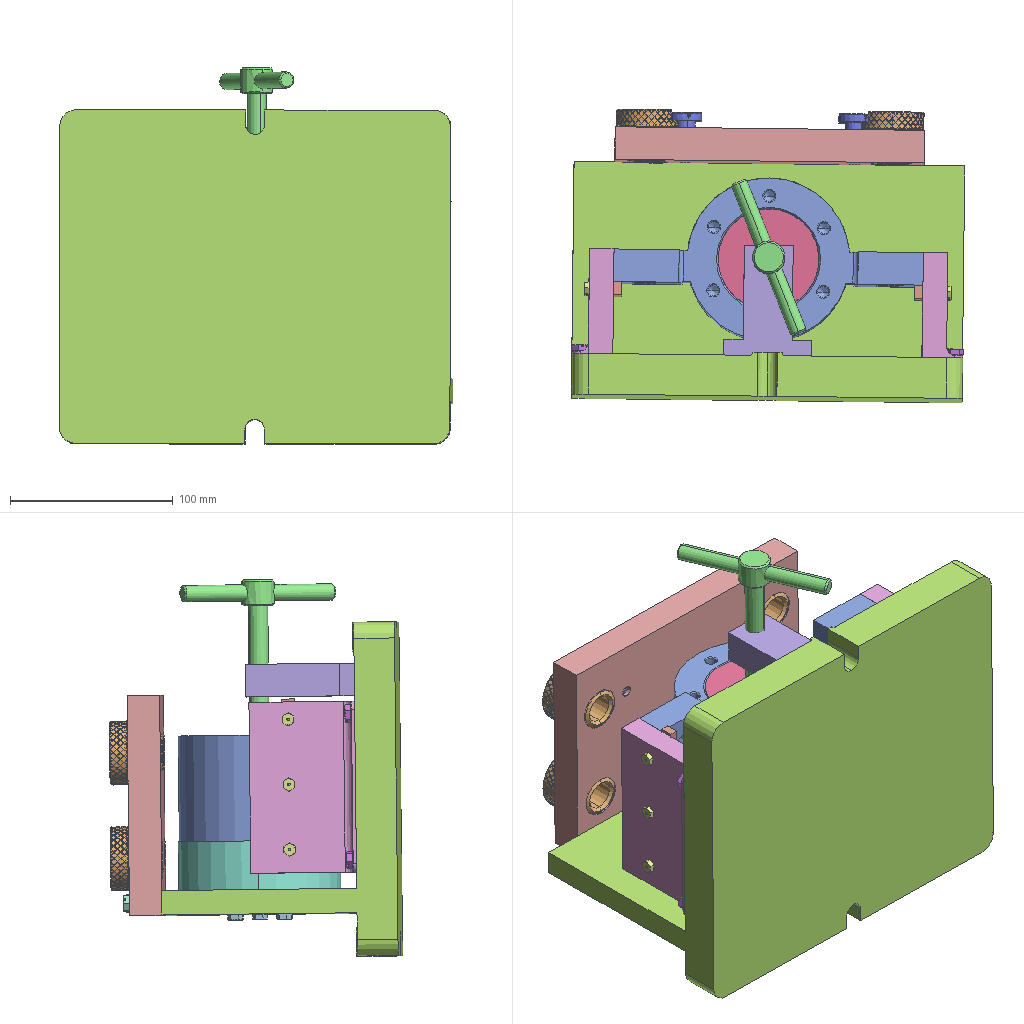Assembly | SolidWorks | 15 different items | 36 placed | box 242 x 180 x 231 mm
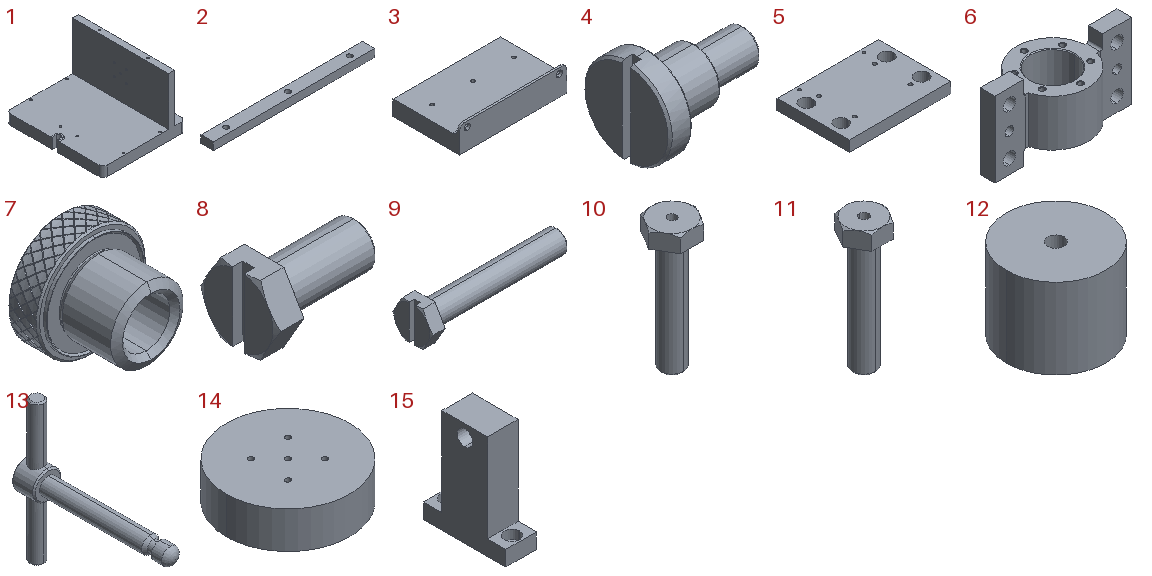Parts list (item | quantity | size | volume | features):
1 | x1 | 205 x 240 x 145 mm | 1648733 mm3 | features HoleWzd 4, Fillet 2, ICE 2, Extrusion 1
2 | x2 | 105 x 8 x 5 mm | 4072 mm3 | features Extrusion 1, HoleWzd 1
3 | x2 | 105 x 65 x 24.968 mm | 104629 mm3 | features Fillet 2, Extrusion 1, HoleWzd 1, ICE 1
4 | x4 | 27 x 20 x 20 mm | 3212 mm3 | features Chamfer 1, Fillet 1, ICE 1, Revolution 1
5 | x1 | 190 x 135 x 20 mm | 469337 mm3 | features HoleWzd 2, Extrusion 1
6 | x1 | 190 x 100 x 105 mm | 479131 mm3 | features ICE 7, Attribute 3, HoleWzd 2, Chamfer 1, Extrusion 1
7 | x4 | 39 x 32 x 39 mm | 16208 mm3 | features Chamfer 2, BlendCut 1, CirPattern 1, ICE 1, MirrorPattern 1, Revolution 1
8 | x4 | 16 x 10.9 x 9.44 mm | 614.542 mm3 | features Cut 2, Chamfer 1, Extrusion 1, Fillet 1, LPattern 1, MoveCopyBody 1, RevCut 1, Revolution 1
9 | x2 | 39 x 10.9 x 9.44 mm | 1265 mm3 | features Cut 2, Chamfer 1, Extrusion 1, Fillet 1, LPattern 1, MoveCopyBody 1, RevCut 1, Revolution 1
10 | x6 | 8.083 x 7 x 22.8 mm | 328.465 mm3 | features ICE 2, Chamfer 1, Revolution 1
11 | x5 | 9.238 x 8 x 28.5 mm | 592.822 mm3 | features ICE 2, Chamfer 1, Revolution 1
12 | x1 | 62 x 62 x 50 mm | 148480 mm3 | features Extrusion 1, HoleWzd 1
13 | x1 | 20 x 106 x 100 mm | 20892 mm3 | features Revolution 5, Chamfer 4, Dome 3
14 | x1 | 100 x 100 x 30 mm | 233541 mm3 | features Extrusion 1, HoleWzd 1
15 | x1 | 20 x 54 x 68 mm | 42750 mm3 | features HoleWzd 2, Extrusion 1, ICE 1
Mates (type | each side: item.copy, entity, surface, feature):
Concentric | 1.1 face cylinder M6 Tapped Hole3 | 3.1 face cylinder Boss-Extrude3 | 2 times
Coincident | 1.1 face plane Boss-Extrude1 | 3.1 face plane Boss-Extrude2
Concentric | 1.1 face cylinder M6 Tapped Hole3 | 3.2 face cylinder Boss-Extrude3 | 2 times
Coincident | 1.1 face plane Boss-Extrude1 | 3.2 face plane Boss-Extrude2
Concentric | 1.1 face cylinder M5 Tapped Hole2 | 14.1 face cylinder M5 Tapped Hole1 | 2 times
Coincident | 1.1 face plane Boss-Extrude5 | 14.1 face plane Boss-Extrude2
Coincident | 6.1 face plane Boss-Extrude1 | 3.2 face plane Boss-Extrude2
Coincident | 6.1 face plane Cut-Extrude2 | 14.1 face plane Boss-Extrude2
Concentric | 5.1 face cylinder M6 Tapped Hole6 | 1.1 face cylinder M6 Tapped Hole6 | 2 times
Coincident | 5.1 face plane Boss-Extrude1 | 1.1 face plane Boss-Extrude5
Concentric | 5.1 face cylinder Boss-Extrude1 | 7.1 face cylinder Revolve1
Parallel | 5.1 face plane Boss-Extrude1 | 7.1 face plane Cut-Extrude1
Concentric | 5.1 face cylinder Boss-Extrude1 | 7.2 face cylinder Revolve1
Coincident | 5.1 face plane Boss-Extrude1 | 7.2 face plane Revolve1
Parallel | 5.1 face plane Boss-Extrude1 | 7.2 face plane Cut-Extrude1
Concentric | 5.1 face cylinder Boss-Extrude1 | 7.3 face cylinder Revolve1
Coincident | 5.1 face plane Boss-Extrude1 | 7.3 face plane Revolve1
Parallel | 5.1 face plane Boss-Extrude1 | 7.3 face plane Cut-Extrude1
Concentric | 5.1 face cylinder Boss-Extrude1 | 7.4 face cylinder Revolve1
Coincident | 5.1 face plane Boss-Extrude1 | 7.4 face plane Revolve1
Parallel | 5.1 face plane Boss-Extrude1 | 7.4 face plane Cut-Extrude1
Concentric | 5.1 face | assembly face
Coincident | assembly face | 7.4 face plane Cut-Extrude1
Concentric | 1.1 face cylinder M6 Tapped Hole7 | 15.1 face cylinder CBORE for M6 Hex Head Bolt1 | 2 times
Coincident | 1.1 face plane Boss-Extrude1 | 15.1 face plane Boss-Extrude1
Concentric | 15.1 face cylinder M12 Tapped Hole1 | 13.1 face cylinder Revolve1
Concentric | 6.1 face cylinder Cut-Extrude5 | 12.1 face cylinder Boss-Extrude1
Coincident | 6.1 face plane Cut-Extrude5 | 12.1 face plane Boss-Extrude1
Concentric | 13.1 face cylinder Revolve5 | 12.1 face cylinder M12 Tapped Hole1
Concentric | 1.1 face cylinder M6 Tapped Hole7 | assembly face | 2 times
Coincident | 15.1 face plane CBORE for M6 Hex Head Bolt1 | assembly face | 2 times
Concentric | 1.1 face cylinder M5 Tapped Hole2 | 11.1 face cylinder Revolve1
Coincident | 1.1 face plane Boss-Extrude5 | 11.1 face plane Boss-Extrude1
Concentric | 1.1 face cylinder M5 Tapped Hole2 | 11.2 face cylinder Revolve1
Coincident | 1.1 face plane Boss-Extrude5 | 11.2 face plane Boss-Extrude1
Concentric | 1.1 face cylinder M5 Tapped Hole2 | 11.3 face cylinder Revolve1
Coincident | 1.1 face plane Boss-Extrude5 | 11.3 face plane Boss-Extrude1
Concentric | 1.1 face cylinder M5 Tapped Hole2 | 11.4 face cylinder Revolve1
Coincident | 1.1 face plane Boss-Extrude5 | 11.4 face plane Boss-Extrude1
Concentric | 1.1 face cylinder M5 Tapped Hole2 | 11.5 face cylinder Revolve1
Coincident | 1.1 face plane Boss-Extrude5 | 11.5 face plane Boss-Extrude1
Concentric | 3.2 face cylinder M4 Tapped Hole2 | 10.1 face cylinder Revolve1
Coincident | 3.2 face plane Boss-Extrude2 | 10.1 face plane Boss-Extrude1
Concentric | 3.2 face cylinder M4 Tapped Hole2 | 10.2 face cylinder Revolve1
Coincident | 3.2 face plane Boss-Extrude2 | 10.2 face plane Boss-Extrude1
Concentric | 3.2 face cylinder M4 Tapped Hole2 | 10.3 face cylinder Revolve1
Coincident | 3.2 face plane Boss-Extrude2 | 10.3 face plane Boss-Extrude1
Concentric | 3.1 face cylinder M4 Tapped Hole2 | 10.4 face cylinder Revolve1
Coincident | 3.1 face plane Boss-Extrude2 | 10.4 face plane Boss-Extrude1
Concentric | 3.1 face cylinder M4 Tapped Hole2 | 10.5 face cylinder Revolve1
Coincident | 3.1 face plane Boss-Extrude2 | 10.5 face plane Boss-Extrude1
Concentric | 3.1 face cylinder M4 Tapped Hole2 | 10.6 face cylinder Revolve1
Coincident | 3.1 face plane Boss-Extrude2 | 10.6 face plane Boss-Extrude1
Concentric | 1.1 face cylinder M6 Tapped Hole3 | 8.1 face cylinder Boss-Revolve1
Coincident | 3.2 face plane Boss-Extrude3 | 8.1 face plane Boss-Revolve1
Concentric | 1.1 face cylinder M6 Tapped Hole3 | 8.2 face cylinder Boss-Revolve1
Coincident | 3.2 face plane Boss-Extrude3 | 8.2 face plane Boss-Revolve1
Concentric | 1.1 face cylinder M6 Tapped Hole3 | 8.3 face cylinder Boss-Revolve1
Coincident | 3.1 face plane Boss-Extrude3 | 8.3 face plane Boss-Revolve1
Concentric | 1.1 face cylinder M6 Tapped Hole3 | 8.4 face cylinder Boss-Revolve1
Coincident | 3.1 face plane Boss-Extrude3 | 8.4 face plane Boss-Revolve1
Concentric | 5.1 face cylinder M6 Tapped Hole6 | 9.1 face cylinder Boss-Revolve1
Coincident | 5.1 face plane Boss-Extrude1 | 9.1 face plane Boss-Revolve1
Concentric | 5.1 face cylinder M6 Tapped Hole6 | 9.2 face cylinder Boss-Revolve1
Coincident | 5.1 face plane Boss-Extrude1 | 9.2 face plane Boss-Revolve1
Concentric | 10.1 face cylinder Revolve1 | 2.1 face cylinder M4 Tapped Hole2
Concentric | 10.3 face cylinder Revolve1 | 2.1 face cylinder M4 Tapped Hole2
Coincident | 3.2 face plane Boss-Extrude2 | 2.1 face plane Boss-Extrude1
Concentric | 10.4 face cylinder Revolve1 | 2.2 face cylinder M4 Tapped Hole2
Concentric | 10.6 face cylinder Revolve1 | 2.2 face cylinder M4 Tapped Hole2
Coincident | 3.1 face plane Boss-Extrude2 | 2.2 face plane Boss-Extrude1
Concentric | 5.1 face cylinder M8 Tapped Hole1 | 4.1 face cylinder Revolve1
Coincident | 7.2 face plane Cut-Extrude1 | 4.1 face plane Revolve1
Concentric | 5.1 face cylinder M8 Tapped Hole1 | 4.2 face cylinder Revolve1
Coincident | 7.1 face plane Cut-Extrude1 | 4.2 face plane Revolve1
Concentric | 5.1 face cylinder M8 Tapped Hole1 | 4.3 face cylinder Revolve1
Coincident | 7.3 face plane Cut-Extrude1 | 4.3 face plane Revolve1
Concentric | 5.1 face cylinder M8 Tapped Hole1 | 4.4 face cylinder Revolve1
Coincident | 7.4 face plane Cut-Extrude1 | 4.4 face plane Revolve1